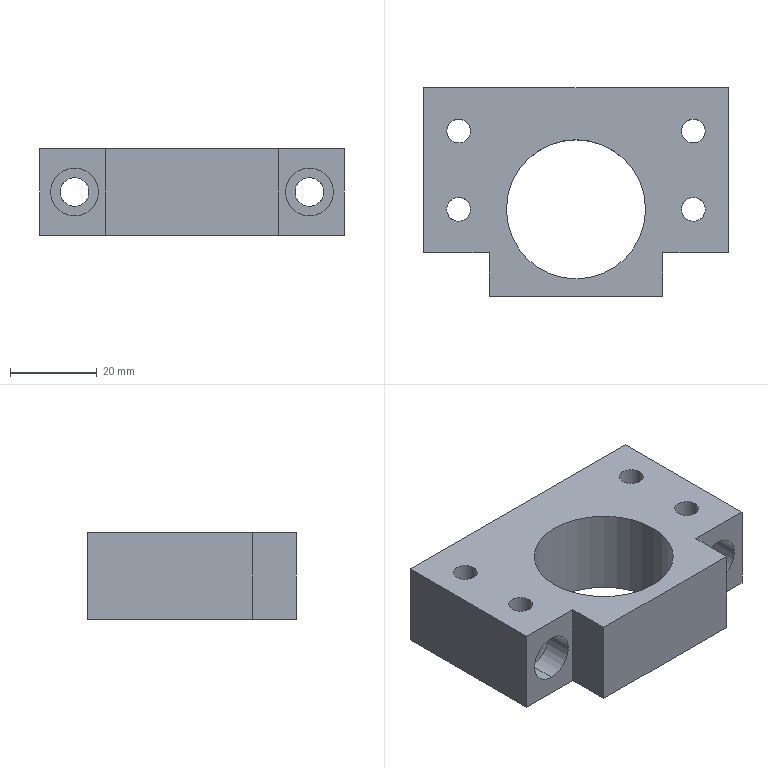Part | SolidWorks | features BaseBody 1 | 1 solid | 38 faces | box 70 x 48 x 20 mm | volume 40390 mm3 | cylinder 26 | plane 12 | commonest cylinder face diameters 5.5 x16 6.6 x4 11 x4 32 x2